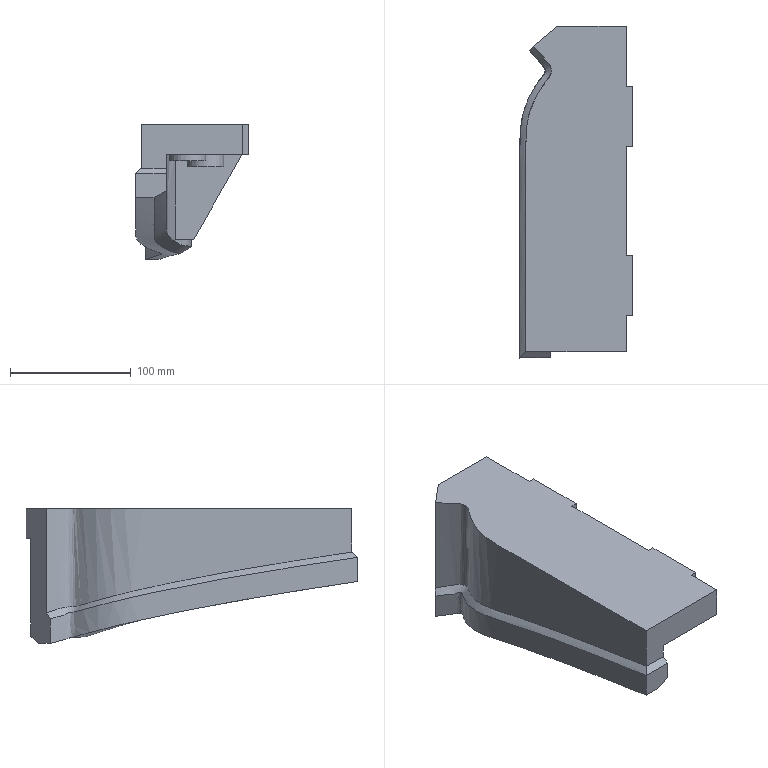Part | NX | features solid 2 | 1 solid | 37 faces | box 93.024 x 275 x 111.795 mm | volume 979391 mm3 | plane 26 | spline 6 | cylinder 5 | commonest cylinder face diameters 30 x5